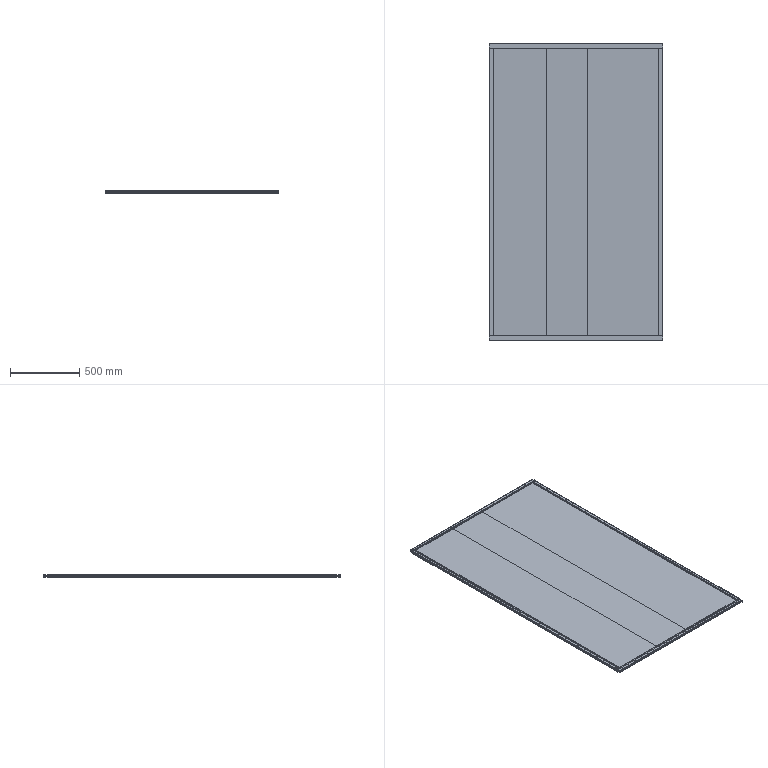Part | SolidWorks | features ICE 3, MirrorPattern 1, WeldMemberFeat 1, WeldmentFeature 1 | 5 solids | 175 faces | box 1250 x 2136 x 18 mm | volume 26549237 mm3 | plane 106 | cylinder 69 | commonest cylinder face diameters 1.1 x24 3.6 x20 5.8 x20 1 x5